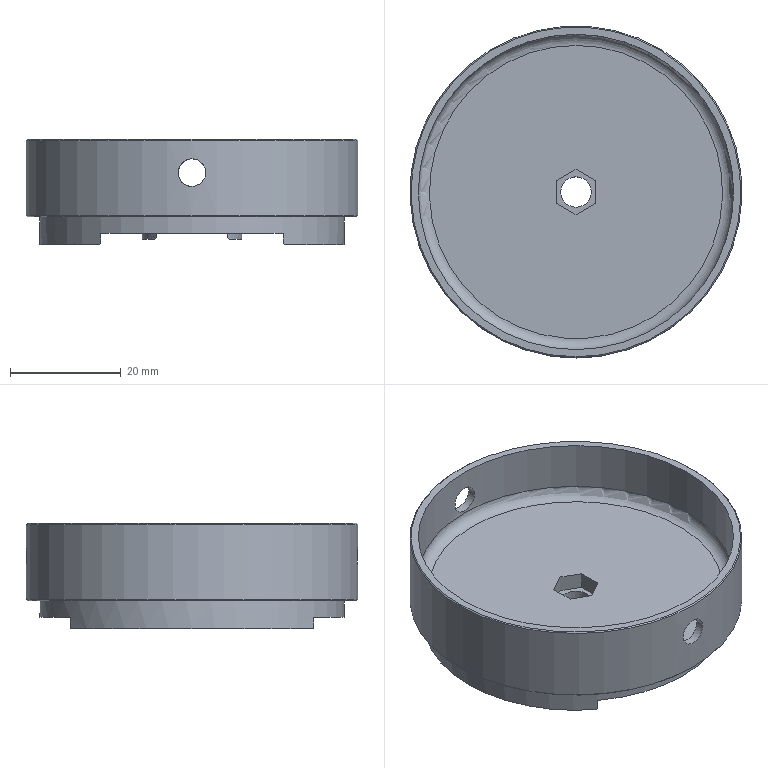NC program | NX | posted with a generic post | part box 60 x 60 x 19 mm
Lines 1 to 296 of 13134:
N10 G17 G21 G94 G90
(FLOOR_WALL_COPY , TOOL : D63)
N12 T01 M6
N14 G54
N16 G17 G0 G90 X-60.792 Y35.721 S1250 M3
N18 G43 Z30. H1
N20 Z7.714
N22 G94 G1 Z4.714 F2200.
N24 X-57.286
N26 X57.286
N28 G2 X59.147 Y32.546 R67.511
N30 X66.037 Y14.025 R67.058
N32 X66.35 Y12.461 R67.511
N34 G1 X-66.353
N36 G3 X-66.901 Y9.047 R67.185
N38 X-67.394 Y3.962 R67.503
N40 X-67.5 Y1.242 R66.868
N42 G1 Y-1.241
N44 G3 X-67.387 Y-4.077 R66.868
N46 X-66.641 Y-10.8 R67.503
N48 G1 X66.642
N50 X69.68
N52 Z7.714
N54 G0 Z30.
N56 X-60.734 Y35.82
N58 Z7.429
N60 G1 Z4.429
N62 X-57.224
N64 X57.224
N66 G2 X61.534 Y27.771 R67.511
N68 X66.341 Y12.51 R67.513
N70 G1 X-66.341
N72 G3 X-67.5 Y1.219 R67.513
N74 G1 Y-1.215
N76 G3 X-66.641 Y-10.8 R67.521
N78 G1 X66.641
N80 X69.679
N82 Z7.429
N84 G0 Z30.
N86 X-60.806 Y35.699
N88 Z7.144
N90 G1 Z4.144
N92 X-57.3
N94 X57.3
N96 G2 X59.328 Y32.215 R67.508
N98 X66.353 Y12.449 R67.513
N100 G1 X-66.353
N102 G3 X-67.5 Y1.219 R67.513
N104 G1 Y-1.215
N106 G3 X-66.641 Y-10.8 R67.521
N108 G1 X66.641
N110 X69.679
N112 Z7.144
N114 G0 Z30.
N116 X-60.735 Y35.819
N118 Z6.859
N120 G1 Z3.859
N122 X-57.225
N124 X57.225
N126 G2 X65.464 Y16.495 R67.508
N128 X66.341 Y12.509 R67.508
N130 G1 X-66.341
N132 G3 X-67.5 Y1.177 R67.508
N134 G1 Y-1.174
N136 G3 X-66.64 Y-10.8 R67.508
N138 G1 X66.641
N140 X69.678
N142 Z6.859
N144 G0 Z30.
N146 X-60.804 Y35.702
N148 Z6.573
N150 G1 Z3.573
N152 X-57.298
N154 X57.301
N156 G2 X66.354 Y12.451 R67.481
N158 G1 X-66.354
N160 G3 X-66.855 Y9.381 R67.275
N162 X-67.5 Y1.17 R67.508
N164 G1 Y-1.185
N166 G3 X-66.642 Y-10.8 R67.441
N168 G1 X66.642
N170 X69.679
N172 Z6.573
N174 G0 Z30.
N176 X-60.742 Y35.816
N178 Z6.288
N180 G1 Z3.288
N182 X-57.231
N184 X57.23
N186 G2 X66.344 Y12.508 R67.481
N188 G1 X-66.346
N190 G3 X-67.5 Y1.368 R67.481
N192 G1 Y-1.345
N194 G3 X-66.692 Y-10.487 R67.481
N196 X-66.642 Y-10.8 R67.441
N198 G1 X66.646
N200 X69.683
N202 Z6.288
N204 G0 Z30.
N206 X-60.741 Y35.817
N208 Z6.003
N210 G1 Z3.003
N212 X-57.231
N214 X57.225
N216 G2 X59.501 Y31.894 R67.506
N218 X60.514 Y29.927 R67.506
N220 X65.023 Y18.156 R67.304
N222 X65.939 Y14.483 R67.506
N224 X66.342 Y12.509 R67.481
N226 G1 X-66.346
N228 G3 X-67.5 Y1.368 R67.481
N230 G1 Y-1.345
N232 G3 X-66.642 Y-10.8 R67.481
N234 G1 X66.646
N236 X69.683
N238 Z6.003
N240 G0 Z30.
N242 X-60.735 Y35.82
N244 Z5.717
N246 G1 Z2.717
N248 X-57.225
N250 X57.224
N252 G2 X66.342 Y12.51 R67.504
N254 G1 X-66.342
N256 G3 X-67.5 Y1.255 R67.486
N258 G1 Y-1.255
N260 G3 X-66.642 Y-10.8 R67.486
N262 G1 X66.641
N264 X69.679
N266 Z5.717
N268 G0 Z30.
N270 X-60.804 Y35.701
N272 Z5.432
N274 G1 Z2.432
N276 X-57.298
N278 X57.298
N280 G2 X66.353 Y12.451 R67.504
N282 G1 X-66.353
N284 G3 X-67.5 Y1.225 R67.496
N286 G1 Y-1.223
N288 G3 X-66.641 Y-10.8 R67.496
N290 G1 X66.641
N292 X69.679
N294 Z5.432
N296 G0 Z30.
N298 X-60.735 Y35.819
N300 Z5.147
N302 G1 Z2.147
N304 X-57.225
N306 X57.225
N308 G2 X62.456 Y25.63 R67.506
N310 X66.341 Y12.51 R67.511
N312 G1 X-66.342
N314 G3 X-67.5 Y1.191 R67.506
N316 G1 Y-1.186
N318 G3 X-66.641 Y-10.8 R67.506
N320 G1 X66.641
N322 X69.679
N324 Z5.147
N326 G0 Z30.
N328 X-60.737 Y35.817
N330 Z4.862
N332 G1 Z1.862
N334 X-57.227
N336 X57.231
N338 G2 X63.46 Y23.031 R67.401
N340 X65.353 Y16.928 R67.506
N342 X66.343 Y12.509 R67.415
N344 G1 X-66.347
N346 G3 X-67.5 Y1.473 R67.415
N348 G1 Y-1.45
N350 G3 X-66.643 Y-10.8 R67.415
N352 G1 X66.647
N354 X69.684
N356 Z4.862
N358 G0 Z30.
N360 X-60.75 Y35.801
N362 Z4.576
N364 G1 Z1.576
N366 X-57.241
N368 X57.241
N370 G2 X62.502 Y25.521 R67.401
N372 X65.992 Y14.239 R67.356
N374 X66.345 Y12.5 R67.415
N376 G1 X-66.349
N378 G3 X-67.5 Y1.473 R67.415
N380 G1 Y-1.45
N382 G3 X-66.643 Y-10.8 R67.415
N384 G1 X66.647
N386 X69.684
N388 Z4.576
N390 G0 Z30.
N392 X-60.801 Y35.715
N394 Z4.291
N396 G1 Z1.291
N398 X-57.294
N400 X57.29
N402 G2 X61.144 Y28.62 R67.502
N404 X66.351 Y12.457 R67.356
N406 G1 X-66.354
N408 G3 X-67.5 Y1.203 R67.473
N410 G1 Y-1.195
N412 G3 X-66.641 Y-10.8 R67.502
N414 G1 X66.643
N416 X69.681
N418 Z4.291
N420 G0 Z30.
N422 X-60.735 Y35.819
N424 Z4.006
N426 G1 Z1.006
N428 X-57.225
N430 X57.225
N432 G2 X62.005 Y26.704 R67.502
N434 X66.342 Y12.51 R67.514
N436 G1 X-66.342
N438 G3 X-66.999 Y8.295 R67.502
N440 X-67.5 Y1.225 R67.514
N442 G1 Y-1.22
N444 G3 X-66.641 Y-10.8 R67.523
N446 G1 X66.641
N448 X69.679
N450 Z4.006
N452 G0 Z30.
N454 X-60.804 Y35.702
N456 Z3.721
N458 G1 Z0.721
N460 X-57.298
N462 X57.298
N464 G2 X66.353 Y12.451 R67.514
N466 G1 X-66.353
N468 G3 X-67.5 Y1.225 R67.514
N470 G1 Y-1.22
N472 G3 X-66.641 Y-10.8 R67.523
N474 G1 X66.641
N476 X69.679
N478 Z3.721
N480 G0 Z30.
N482 X-60.807 Y35.697
N484 Z3.435
N486 G1 Z0.435
N488 X-57.302
N490 X57.301
N492 G2 X62.31 Y25.984 R67.506
N494 X66.353 Y12.449 R67.511
N496 G1 X-66.353
N498 G3 X-67.5 Y1.192 R67.506
N500 G1 Y-1.187
N502 G3 X-66.641 Y-10.8 R67.506
N504 G1 X66.641
N506 X69.679
N508 Z3.435
N510 G0 Z30.
N512 X-60.736 Y35.818
N514 Z3.15
N516 G1 Z0.15
N518 X-57.226
N520 X57.225
N522 G2 X61.956 Y26.815 R67.506
N524 X66.341 Y12.509 R67.508
N526 G1 X-66.342
N528 G3 X-67.5 Y1.21 R67.504
N530 G1 Y-1.206
N532 G3 X-66.641 Y-10.8 R67.504
N534 G1 X66.641
N536 X69.679
N538 Z3.15
N540 G0 Z30.
(FLOOR_WALL_COPY_1 , TOOL : D63)
N542 X-60.791 Y35.718 S1200
N544 Z3.
N546 G1 Z0. F1250.
N548 X-57.284
N550 X57.286
N552 G2 X57.955 Y34.619 R67.32
N554 X60.276 Y30.409 R67.074
N556 X66.349 Y12.459 R67.058
N558 G1 X-66.353
N560 G3 X-67.039 Y7.96 R67.185
N562 X-67.171 Y6.739 R67.234
N564 X-67.491 Y1.666 R66.889
N566 X-67.5 Y1.242 R66.868
N568 G1 Y-1.241
N570 G3 X-67.183 Y-6.618 R66.868
N572 X-66.813 Y-9.641 R66.889
N574 X-66.639 Y-10.8 R66.093
N576 G1 X66.642
N578 X69.68
N580 Z3.
N582 G0 Z30.
N584 M5